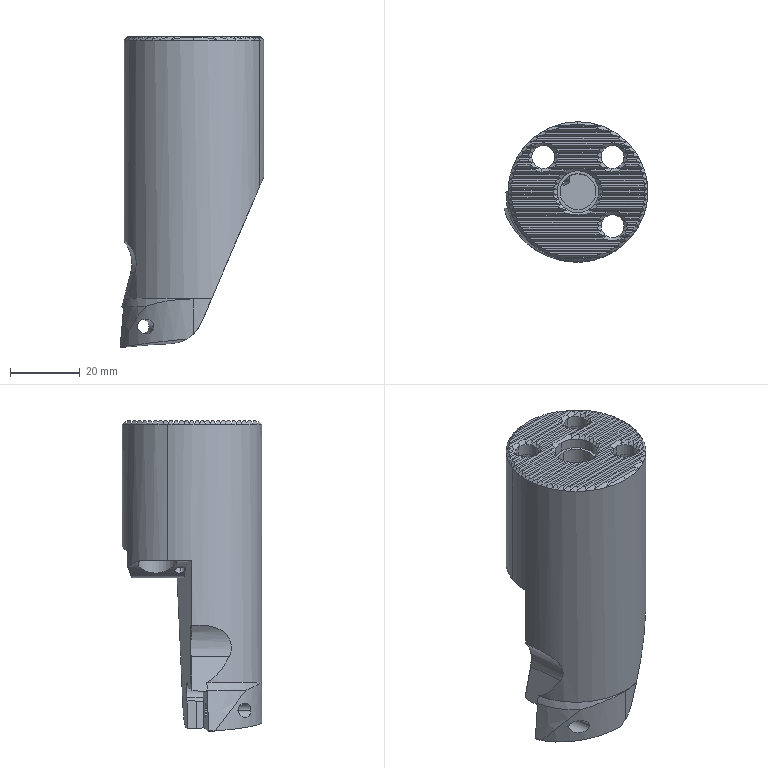Part | 1 solid | 218 faces | volume 59531 mm3 | plane 174 | cylinder 30 | cone 13 | torus 1 | commonest cylinder face diameters 6.6 x6 11 x6 2.9 x2 4.2 x2 10.3 x2 12 x2